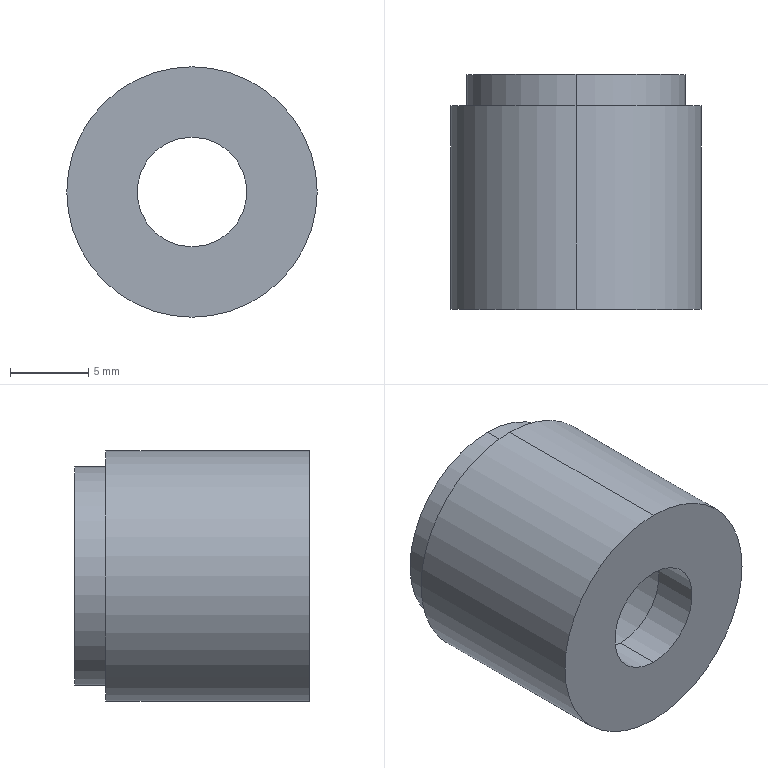Part | STEP file | Generic block | 1 solid | 12 faces | box 16 x 15 x 16 mm | volume 1666 mm3 | cylinder 8 | plane 4 | commonest cylinder face diameters 7 x2 11 x2 14 x2 16 x2
STEP:
#1=CARTESIAN_POINT('',(0.,0.,0.));
#2=DIRECTION('',(0.,0.,1.));
#3=DIRECTION('',(1.,0.,0.));
#4=AXIS2_PLACEMENT_3D('',#1,#2,#3);
#5=CARTESIAN_POINT('',(3.5,3.,5.5));
#6=VERTEX_POINT('',#5);
#7=CARTESIAN_POINT('',(3.5,15.,5.5));
#8=VERTEX_POINT('',#7);
#9=CARTESIAN_POINT('',(3.5,3.,5.5));
#10=DIRECTION('',(0.,1.,0.));
#11=VECTOR('',#10,1.);
#12=LINE('',#9,#11);
#13=CARTESIAN_POINT('',(3.5,3.,0.));
#14=DIRECTION('',(0.,1.,0.));
#15=DIRECTION('',(0.,0.,1.));
#16=AXIS2_PLACEMENT_3D('',#13,#14,#15);
#17=CYLINDRICAL_SURFACE('',#16,5.5);
#18=CARTESIAN_POINT('',(6.283,0.));
#19=DIRECTION('',(0.,1.));
#20=VECTOR('',#19,1.);
#21=LINE('',#18,#20);
#22=(GEOMETRIC_REPRESENTATION_CONTEXT(2)PARAMETRIC_REPRESENTATION_CONTEXT()REPRESENTATION_CONTEXT('',''));
#23=DEFINITIONAL_REPRESENTATION('',(#21),#22);
#24=PCURVE('',#17,#23);
#25=CARTESIAN_POINT('',(3.5,3.,0.));
#26=DIRECTION('',(0.,1.,0.));
#27=DIRECTION('',(0.,0.,1.));
#28=AXIS2_PLACEMENT_3D('',#25,#26,#27);
#29=CYLINDRICAL_SURFACE('',#28,5.5);
#30=CARTESIAN_POINT('',(0.,0.));
#31=DIRECTION('',(0.,1.));
#32=VECTOR('',#31,1.);
#33=LINE('',#30,#32);
#34=(GEOMETRIC_REPRESENTATION_CONTEXT(2)PARAMETRIC_REPRESENTATION_CONTEXT()REPRESENTATION_CONTEXT('',''));
#35=DEFINITIONAL_REPRESENTATION('',(#33),#34);
#36=PCURVE('',#29,#35);
#37=SURFACE_CURVE('',#12,(#24,#36),.PCURVE_S1.);
#38=EDGE_CURVE('',#6,#8,#37,.T.);
#39=ORIENTED_EDGE('',*,*,#38,.T.);
#40=CARTESIAN_POINT('',(3.5,15.,-5.5));
#41=VERTEX_POINT('',#40);
#42=CARTESIAN_POINT('',(3.5,15.,0.));
#43=DIRECTION('',(0.,1.,0.));
#44=DIRECTION('',(0.,0.,1.));
#45=AXIS2_PLACEMENT_3D('',#42,#43,#44);
#46=CIRCLE('',#45,5.5);
#47=CARTESIAN_POINT('',(0.,12.));
#48=DIRECTION('',(1.,0.));
#49=VECTOR('',#48,1.);
#50=LINE('',#47,#49);
#51=(GEOMETRIC_REPRESENTATION_CONTEXT(2)PARAMETRIC_REPRESENTATION_CONTEXT()REPRESENTATION_CONTEXT('',''));
#52=DEFINITIONAL_REPRESENTATION('',(#50),#51);
#53=PCURVE('',#17,#52);
#54=CARTESIAN_POINT('',(-3.5,15.,0.));
#55=DIRECTION('',(0.,-1.,0.));
#56=DIRECTION('',(0.,0.,-1.));
#57=AXIS2_PLACEMENT_3D('',#54,#55,#56);
#58=PLANE('',#57);
#59=CARTESIAN_POINT('',(-5.5,7.));
#60=CARTESIAN_POINT('',(-5.5,16.526));
#61=CARTESIAN_POINT('',(2.75,11.763));
#62=CARTESIAN_POINT('',(11.,7.));
#63=CARTESIAN_POINT('',(2.75,2.237));
#64=CARTESIAN_POINT('',(-5.5,-2.526));
#65=CARTESIAN_POINT('',(-5.5,7.));
#66=(BOUNDED_CURVE()B_SPLINE_CURVE(2,(#59,#60,#61,#62,#63,#64,#65),.UNSPECIFIED.,.T.,.F.)B_SPLINE_CURVE_WITH_KNOTS((1,2,2,2,2,1),(-2.094,0.,2.094,4.189,6.283,8.378),.UNSPECIFIED.)CURVE()GEOMETRIC_REPRESENTATION_ITEM()RATIONAL_B_SPLINE_CURVE((1.,0.5,1.,0.5,1.,0.5,1.))REPRESENTATION_ITEM(''));
#67=(GEOMETRIC_REPRESENTATION_CONTEXT(2)PARAMETRIC_REPRESENTATION_CONTEXT()REPRESENTATION_CONTEXT('',''));
#68=DEFINITIONAL_REPRESENTATION('',(#66),#67);
#69=PCURVE('',#58,#68);
#70=SURFACE_CURVE('',#46,(#53,#69),.PCURVE_S1.);
#71=EDGE_CURVE('',#41,#8,#70,.T.);
#72=ORIENTED_EDGE('',*,*,#71,.F.);
#73=CARTESIAN_POINT('',(3.5,3.,-5.5));
#74=VERTEX_POINT('',#73);
#75=CARTESIAN_POINT('',(3.5,3.,-5.5));
#76=DIRECTION('',(0.,1.,0.));
#77=VECTOR('',#76,1.);
#78=LINE('',#75,#77);
#79=CARTESIAN_POINT('',(3.142,0.));
#80=DIRECTION('',(0.,1.));
#81=VECTOR('',#80,1.);
#82=LINE('',#79,#81);
#83=(GEOMETRIC_REPRESENTATION_CONTEXT(2)PARAMETRIC_REPRESENTATION_CONTEXT()REPRESENTATION_CONTEXT('',''));
#84=DEFINITIONAL_REPRESENTATION('',(#82),#83);
#85=PCURVE('',#17,#84);
#86=CARTESIAN_POINT('',(3.142,0.));
#87=DIRECTION('',(0.,1.));
#88=VECTOR('',#87,1.);
#89=LINE('',#86,#88);
#90=(GEOMETRIC_REPRESENTATION_CONTEXT(2)PARAMETRIC_REPRESENTATION_CONTEXT()REPRESENTATION_CONTEXT('',''));
#91=DEFINITIONAL_REPRESENTATION('',(#89),#90);
#92=PCURVE('',#29,#91);
#93=SURFACE_CURVE('',#78,(#85,#92),.PCURVE_S1.);
#94=EDGE_CURVE('',#74,#41,#93,.T.);
#95=ORIENTED_EDGE('',*,*,#94,.F.);
#96=CARTESIAN_POINT('',(3.5,3.,0.));
#97=DIRECTION('',(0.,1.,0.));
#98=DIRECTION('',(0.,0.,1.));
#99=AXIS2_PLACEMENT_3D('',#96,#97,#98);
#100=CIRCLE('',#99,5.5);
#101=CARTESIAN_POINT('',(0.,0.));
#102=DIRECTION('',(1.,0.));
#103=VECTOR('',#102,1.);
#104=LINE('',#101,#103);
#105=(GEOMETRIC_REPRESENTATION_CONTEXT(2)PARAMETRIC_REPRESENTATION_CONTEXT()REPRESENTATION_CONTEXT('',''));
#106=DEFINITIONAL_REPRESENTATION('',(#104),#105);
#107=PCURVE('',#17,#106);
#108=CARTESIAN_POINT('',(3.5,3.,0.));
#109=DIRECTION('',(0.,1.,0.));
#110=DIRECTION('',(0.,0.,1.));
#111=AXIS2_PLACEMENT_3D('',#108,#109,#110);
#112=PLANE('',#111);
#113=CARTESIAN_POINT('',(0.,0.));
#114=DIRECTION('',(1.,0.));
#115=AXIS2_PLACEMENT_2D('',#113,#114);
#116=CIRCLE('',#115,5.5);
#117=(GEOMETRIC_REPRESENTATION_CONTEXT(2)PARAMETRIC_REPRESENTATION_CONTEXT()REPRESENTATION_CONTEXT('',''));
#118=DEFINITIONAL_REPRESENTATION('',(#116),#117);
#119=PCURVE('',#112,#118);
#120=SURFACE_CURVE('',#100,(#107,#119),.PCURVE_S1.);
#121=EDGE_CURVE('',#74,#6,#120,.T.);
#122=ORIENTED_EDGE('',*,*,#121,.T.);
#123=EDGE_LOOP('',(#39,#72,#95,#122));
#124=FACE_BOUND('',#123,.F.);
#125=ADVANCED_FACE('',(#124),#17,.F.);
#126=CARTESIAN_POINT('',(3.5,15.,-7.));
#127=VERTEX_POINT('',#126);
#128=CARTESIAN_POINT('',(3.5,15.,7.));
#129=VERTEX_POINT('',#128);
#130=CARTESIAN_POINT('',(3.5,15.,0.));
#131=DIRECTION('',(0.,-1.,0.));
#132=DIRECTION('',(0.,0.,-1.));
#133=AXIS2_PLACEMENT_3D('',#130,#131,#132);
#134=CIRCLE('',#133,7.);
#135=CARTESIAN_POINT('',(3.5,0.,0.));
#136=DIRECTION('',(0.,-1.,0.));
#137=DIRECTION('',(0.,0.,-1.));
#138=AXIS2_PLACEMENT_3D('',#135,#136,#137);
#139=CYLINDRICAL_SURFACE('',#138,7.);
#140=CARTESIAN_POINT('',(0.,-15.));
#141=DIRECTION('',(1.,0.));
#142=VECTOR('',#141,1.);
#143=LINE('',#140,#142);
#144=(GEOMETRIC_REPRESENTATION_CONTEXT(2)PARAMETRIC_REPRESENTATION_CONTEXT()REPRESENTATION_CONTEXT('',''));
#145=DEFINITIONAL_REPRESENTATION('',(#143),#144);
#146=PCURVE('',#139,#145);
#147=CARTESIAN_POINT('',(0.,7.));
#148=DIRECTION('',(1.,0.));
#149=AXIS2_PLACEMENT_2D('',#147,#148);
#150=CIRCLE('',#149,7.);
#151=(GEOMETRIC_REPRESENTATION_CONTEXT(2)PARAMETRIC_REPRESENTATION_CONTEXT()REPRESENTATION_CONTEXT('',''));
#152=DEFINITIONAL_REPRESENTATION('',(#150),#151);
#153=PCURVE('',#58,#152);
#154=SURFACE_CURVE('',#134,(#146,#153),.PCURVE_S1.);
#155=EDGE_CURVE('',#127,#129,#154,.T.);
#156=ORIENTED_EDGE('',*,*,#155,.T.);
#157=CARTESIAN_POINT('',(3.5,13.,7.));
#158=VERTEX_POINT('',#157);
#159=CARTESIAN_POINT('',(3.5,0.,7.));
#160=DIRECTION('',(0.,-1.,0.));
#161=VECTOR('',#160,1.);
#162=LINE('',#159,#161);
#163=CARTESIAN_POINT('',(3.142,0.));
#164=DIRECTION('',(0.,1.));
#165=VECTOR('',#164,1.);
#166=LINE('',#163,#165);
#167=(GEOMETRIC_REPRESENTATION_CONTEXT(2)PARAMETRIC_REPRESENTATION_CONTEXT()REPRESENTATION_CONTEXT('',''));
#168=DEFINITIONAL_REPRESENTATION('',(#166),#167);
#169=PCURVE('',#139,#168);
#170=CARTESIAN_POINT('',(3.5,0.,0.));
#171=DIRECTION('',(0.,-1.,0.));
#172=DIRECTION('',(0.,0.,-1.));
#173=AXIS2_PLACEMENT_3D('',#170,#171,#172);
#174=CYLINDRICAL_SURFACE('',#173,7.);
#175=CARTESIAN_POINT('',(3.142,0.));
#176=DIRECTION('',(0.,1.));
#177=VECTOR('',#176,1.);
#178=LINE('',#175,#177);
#179=(GEOMETRIC_REPRESENTATION_CONTEXT(2)PARAMETRIC_REPRESENTATION_CONTEXT()REPRESENTATION_CONTEXT('',''));
#180=DEFINITIONAL_REPRESENTATION('',(#178),#179);
#181=PCURVE('',#174,#180);
#182=SURFACE_CURVE('',#162,(#169,#181),.PCURVE_S1.);
#183=EDGE_CURVE('',#129,#158,#182,.T.);
#184=ORIENTED_EDGE('',*,*,#183,.T.);
#185=CARTESIAN_POINT('',(3.5,13.,-7.));
#186=VERTEX_POINT('',#185);
#187=CARTESIAN_POINT('',(3.5,13.,0.));
#188=DIRECTION('',(0.,-1.,0.));
#189=DIRECTION('',(0.,0.,-1.));
#190=AXIS2_PLACEMENT_3D('',#187,#188,#189);
#191=CIRCLE('',#190,7.);
#192=CARTESIAN_POINT('',(0.,-13.));
#193=DIRECTION('',(1.,0.));
#194=VECTOR('',#193,1.);
#195=LINE('',#192,#194);
#196=(GEOMETRIC_REPRESENTATION_CONTEXT(2)PARAMETRIC_REPRESENTATION_CONTEXT()REPRESENTATION_CONTEXT('',''));
#197=DEFINITIONAL_REPRESENTATION('',(#195),#196);
#198=PCURVE('',#139,#197);
#199=CARTESIAN_POINT('',(-4.5,13.,0.));
#200=DIRECTION('',(0.,-1.,0.));
#201=DIRECTION('',(0.,0.,-1.));
#202=AXIS2_PLACEMENT_3D('',#199,#200,#201);
#203=PLANE('',#202);
#204=CARTESIAN_POINT('',(0.,8.));
#205=DIRECTION('',(1.,0.));
#206=AXIS2_PLACEMENT_2D('',#204,#205);
#207=CIRCLE('',#206,7.);
#208=(GEOMETRIC_REPRESENTATION_CONTEXT(2)PARAMETRIC_REPRESENTATION_CONTEXT()REPRESENTATION_CONTEXT('',''));
#209=DEFINITIONAL_REPRESENTATION('',(#207),#208);
#210=PCURVE('',#203,#209);
#211=SURFACE_CURVE('',#191,(#198,#210),.PCURVE_S1.);
#212=EDGE_CURVE('',#186,#158,#211,.T.);
#213=ORIENTED_EDGE('',*,*,#212,.F.);
#214=CARTESIAN_POINT('',(3.5,0.,-7.));
#215=DIRECTION('',(0.,-1.,0.));
#216=VECTOR('',#215,1.);
#217=LINE('',#214,#216);
#218=CARTESIAN_POINT('',(0.,0.));
#219=DIRECTION('',(0.,1.));
#220=VECTOR('',#219,1.);
#221=LINE('',#218,#220);
#222=(GEOMETRIC_REPRESENTATION_CONTEXT(2)PARAMETRIC_REPRESENTATION_CONTEXT()REPRESENTATION_CONTEXT('',''));
#223=DEFINITIONAL_REPRESENTATION('',(#221),#222);
#224=PCURVE('',#139,#223);
#225=CARTESIAN_POINT('',(6.283,0.));
#226=DIRECTION('',(0.,1.));
#227=VECTOR('',#226,1.);
#228=LINE('',#225,#227);
#229=(GEOMETRIC_REPRESENTATION_CONTEXT(2)PARAMETRIC_REPRESENTATION_CONTEXT()REPRESENTATION_CONTEXT('',''));
#230=DEFINITIONAL_REPRESENTATION('',(#228),#229);
#231=PCURVE('',#174,#230);
#232=SURFACE_CURVE('',#217,(#224,#231),.PCURVE_S1.);
#233=EDGE_CURVE('',#127,#186,#232,.T.);
#234=ORIENTED_EDGE('',*,*,#233,.F.);
#235=EDGE_LOOP('',(#156,#184,#213,#234));
#236=FACE_BOUND('',#235,.T.);
#237=ADVANCED_FACE('',(#236),#139,.T.);
#238=CARTESIAN_POINT('',(3.5,13.,-8.));
#239=VERTEX_POINT('',#238);
#240=CARTESIAN_POINT('',(3.5,13.,8.));
#241=VERTEX_POINT('',#240);
#242=CARTESIAN_POINT('',(3.5,13.,0.));
#243=DIRECTION('',(0.,-1.,0.));
#244=DIRECTION('',(0.,0.,-1.));
#245=AXIS2_PLACEMENT_3D('',#242,#243,#244);
#246=CIRCLE('',#245,8.);
#247=CARTESIAN_POINT('',(3.5,0.,0.));
#248=DIRECTION('',(0.,-1.,0.));
#249=DIRECTION('',(0.,0.,-1.));
#250=AXIS2_PLACEMENT_3D('',#247,#248,#249);
#251=CYLINDRICAL_SURFACE('',#250,8.);
#252=CARTESIAN_POINT('',(0.,-13.));
#253=DIRECTION('',(1.,0.));
#254=VECTOR('',#253,1.);
#255=LINE('',#252,#254);
#256=(GEOMETRIC_REPRESENTATION_CONTEXT(2)PARAMETRIC_REPRESENTATION_CONTEXT()REPRESENTATION_CONTEXT('',''));
#257=DEFINITIONAL_REPRESENTATION('',(#255),#256);
#258=PCURVE('',#251,#257);
#259=CARTESIAN_POINT('',(0.,8.));
#260=DIRECTION('',(1.,0.));
#261=AXIS2_PLACEMENT_2D('',#259,#260);
#262=CIRCLE('',#261,8.);
#263=(GEOMETRIC_REPRESENTATION_CONTEXT(2)PARAMETRIC_REPRESENTATION_CONTEXT()REPRESENTATION_CONTEXT('',''));
#264=DEFINITIONAL_REPRESENTATION('',(#262),#263);
#265=PCURVE('',#203,#264);
#266=SURFACE_CURVE('',#246,(#258,#265),.PCURVE_S1.);
#267=EDGE_CURVE('',#239,#241,#266,.T.);
#268=ORIENTED_EDGE('',*,*,#267,.T.);
#269=CARTESIAN_POINT('',(3.5,0.,8.));
#270=VERTEX_POINT('',#269);
#271=CARTESIAN_POINT('',(3.5,0.,8.));
#272=DIRECTION('',(0.,-1.,0.));
#273=VECTOR('',#272,1.);
#274=LINE('',#271,#273);
#275=CARTESIAN_POINT('',(3.142,0.));
#276=DIRECTION('',(0.,1.));
#277=VECTOR('',#276,1.);
#278=LINE('',#275,#277);
#279=(GEOMETRIC_REPRESENTATION_CONTEXT(2)PARAMETRIC_REPRESENTATION_CONTEXT()REPRESENTATION_CONTEXT('',''));
#280=DEFINITIONAL_REPRESENTATION('',(#278),#279);
#281=PCURVE('',#251,#280);
#282=CARTESIAN_POINT('',(3.5,0.,0.));
#283=DIRECTION('',(0.,-1.,0.));
#284=DIRECTION('',(0.,0.,-1.));
#285=AXIS2_PLACEMENT_3D('',#282,#283,#284);
#286=CYLINDRICAL_SURFACE('',#285,8.);
#287=CARTESIAN_POINT('',(3.142,0.));
#288=DIRECTION('',(0.,1.));
#289=VECTOR('',#288,1.);
#290=LINE('',#287,#289);
#291=(GEOMETRIC_REPRESENTATION_CONTEXT(2)PARAMETRIC_REPRESENTATION_CONTEXT()REPRESENTATION_CONTEXT('',''));
#292=DEFINITIONAL_REPRESENTATION('',(#290),#291);
#293=PCURVE('',#286,#292);
#294=SURFACE_CURVE('',#274,(#281,#293),.PCURVE_S1.);
#295=EDGE_CURVE('',#241,#270,#294,.T.);
#296=ORIENTED_EDGE('',*,*,#295,.T.);
#297=CARTESIAN_POINT('',(3.5,0.,-8.));
#298=VERTEX_POINT('',#297);
#299=CARTESIAN_POINT('',(3.5,0.,0.));
#300=DIRECTION('',(0.,-1.,0.));
#301=DIRECTION('',(0.,0.,-1.));
#302=AXIS2_PLACEMENT_3D('',#299,#300,#301);
#303=CIRCLE('',#302,8.);
#304=CARTESIAN_POINT('',(0.,0.));
#305=DIRECTION('',(1.,0.));
#306=VECTOR('',#305,1.);
#307=LINE('',#304,#306);
#308=(GEOMETRIC_REPRESENTATION_CONTEXT(2)PARAMETRIC_REPRESENTATION_CONTEXT()REPRESENTATION_CONTEXT('',''));
#309=DEFINITIONAL_REPRESENTATION('',(#307),#308);
#310=PCURVE('',#251,#309);
#311=CARTESIAN_POINT('',(0.,0.,0.));
#312=DIRECTION('',(0.,1.,0.));
#313=DIRECTION('',(0.,0.,1.));
#314=AXIS2_PLACEMENT_3D('',#311,#312,#313);
#315=PLANE('',#314);
#316=CARTESIAN_POINT('',(-8.,3.5));
#317=CARTESIAN_POINT('',(-8.,17.356));
#318=CARTESIAN_POINT('',(4.,10.428));
#319=CARTESIAN_POINT('',(16.,3.5));
#320=CARTESIAN_POINT('',(4.,-3.428));
#321=CARTESIAN_POINT('',(-8.,-10.356));
#322=CARTESIAN_POINT('',(-8.,3.5));
#323=(BOUNDED_CURVE()B_SPLINE_CURVE(2,(#316,#317,#318,#319,#320,#321,#322),.UNSPECIFIED.,.T.,.F.)B_SPLINE_CURVE_WITH_KNOTS((1,2,2,2,2,1),(-2.094,0.,2.094,4.189,6.283,8.378),.UNSPECIFIED.)CURVE()GEOMETRIC_REPRESENTATION_ITEM()RATIONAL_B_SPLINE_CURVE((1.,0.5,1.,0.5,1.,0.5,1.))REPRESENTATION_ITEM(''));
#324=(GEOMETRIC_REPRESENTATION_CONTEXT(2)PARAMETRIC_REPRESENTATION_CONTEXT()REPRESENTATION_CONTEXT('',''));
#325=DEFINITIONAL_REPRESENTATION('',(#323),#324);
#326=PCURVE('',#315,#325);
#327=SURFACE_CURVE('',#303,(#310,#326),.PCURVE_S1.);
#328=EDGE_CURVE('',#298,#270,#327,.T.);
#329=ORIENTED_EDGE('',*,*,#328,.F.);
#330=CARTESIAN_POINT('',(3.5,0.,-8.));
#331=DIRECTION('',(0.,-1.,0.));
#332=VECTOR('',#331,1.);
#333=LINE('',#330,#332);
#334=CARTESIAN_POINT('',(0.,0.));
#335=DIRECTION('',(0.,1.));
#336=VECTOR('',#335,1.);
#337=LINE('',#334,#336);
#338=(GEOMETRIC_REPRESENTATION_CONTEXT(2)PARAMETRIC_REPRESENTATION_CONTEXT()REPRESENTATION_CONTEXT('',''));
#339=DEFINITIONAL_REPRESENTATION('',(#337),#338);
#340=PCURVE('',#251,#339);
#341=CARTESIAN_POINT('',(6.283,0.));
#342=DIRECTION('',(0.,1.));
#343=VECTOR('',#342,1.);
#344=LINE('',#341,#343);
#345=(GEOMETRIC_REPRESENTATION_CONTEXT(2)PARAMETRIC_REPRESENTATION_CONTEXT()REPRESENTATION_CONTEXT('',''));
#346=DEFINITIONAL_REPRESENTATION('',(#344),#345);
#347=PCURVE('',#286,#346);
#348=SURFACE_CURVE('',#333,(#340,#347),.PCURVE_S1.);
#349=EDGE_CURVE('',#239,#298,#348,.T.);
#350=ORIENTED_EDGE('',*,*,#349,.F.);
#351=EDGE_LOOP('',(#268,#296,#329,#350));
#352=FACE_BOUND('',#351,.T.);
#353=ADVANCED_FACE('',(#352),#251,.T.);
#354=CARTESIAN_POINT('',(3.5,3.,-3.5));
#355=VERTEX_POINT('',#354);
#356=CARTESIAN_POINT('',(3.5,0.,-3.5));
#357=VERTEX_POINT('',#356);
#358=CARTESIAN_POINT('',(3.5,0.,-3.5));
#359=DIRECTION('',(0.,-1.,0.));
#360=VECTOR('',#359,1.);
#361=LINE('',#358,#360);
#362=CARTESIAN_POINT('',(3.5,0.,0.));
#363=DIRECTION('',(0.,-1.,0.));
#364=DIRECTION('',(0.,0.,-1.));
#365=AXIS2_PLACEMENT_3D('',#362,#363,#364);
#366=CYLINDRICAL_SURFACE('',#365,3.5);
#367=CARTESIAN_POINT('',(6.283,0.));
#368=DIRECTION('',(0.,1.));
#369=VECTOR('',#368,1.);
#370=LINE('',#367,#369);
#371=(GEOMETRIC_REPRESENTATION_CONTEXT(2)PARAMETRIC_REPRESENTATION_CONTEXT()REPRESENTATION_CONTEXT('',''));
#372=DEFINITIONAL_REPRESENTATION('',(#370),#371);
#373=PCURVE('',#366,#372);
#374=CARTESIAN_POINT('',(3.5,0.,0.));
#375=DIRECTION('',(0.,-1.,0.));
#376=DIRECTION('',(0.,0.,-1.));
#377=AXIS2_PLACEMENT_3D('',#374,#375,#376);
#378=CYLINDRICAL_SURFACE('',#377,3.5);
#379=CARTESIAN_POINT('',(0.,0.));
#380=DIRECTION('',(0.,1.));
#381=VECTOR('',#380,1.);
#382=LINE('',#379,#381);
#383=(GEOMETRIC_REPRESENTATION_CONTEXT(2)PARAMETRIC_REPRESENTATION_CONTEXT()REPRESENTATION_CONTEXT('',''));
#384=DEFINITIONAL_REPRESENTATION('',(#382),#383);
#385=PCURVE('',#378,#384);
#386=SURFACE_CURVE('',#361,(#373,#385),.PCURVE_S1.);
#387=EDGE_CURVE('',#355,#357,#386,.T.);
#388=ORIENTED_EDGE('',*,*,#387,.T.);
#389=CARTESIAN_POINT('',(3.5,0.,3.5));
#390=VERTEX_POINT('',#389);
#391=CARTESIAN_POINT('',(3.5,0.,0.));
#392=DIRECTION('',(0.,-1.,0.));
#393=DIRECTION('',(0.,0.,-1.));
#394=AXIS2_PLACEMENT_3D('',#391,#392,#393);
#395=CIRCLE('',#394,3.5);
#396=CARTESIAN_POINT('',(0.,0.));
#397=DIRECTION('',(1.,0.));
#398=VECTOR('',#397,1.);
#399=LINE('',#396,#398);
#400=(GEOMETRIC_REPRESENTATION_CONTEXT(2)PARAMETRIC_REPRESENTATION_CONTEXT()REPRESENTATION_CONTEXT('',''));
#401=DEFINITIONAL_REPRESENTATION('',(#399),#400);
#402=PCURVE('',#366,#401);
#403=CARTESIAN_POINT('',(-3.5,3.5));
#404=CARTESIAN_POINT('',(-3.5,9.562));
#405=CARTESIAN_POINT('',(1.75,6.531));
#406=CARTESIAN_POINT('',(7.,3.5));
#407=CARTESIAN_POINT('',(1.75,0.4689));
#408=CARTESIAN_POINT('',(-3.5,-2.562));
#409=CARTESIAN_POINT('',(-3.5,3.5));
#410=(BOUNDED_CURVE()B_SPLINE_CURVE(2,(#403,#404,#405,#406,#407,#408,#409),.UNSPECIFIED.,.T.,.F.)B_SPLINE_CURVE_WITH_KNOTS((1,2,2,2,2,1),(-2.094,0.,2.094,4.189,6.283,8.378),.UNSPECIFIED.)CURVE()GEOMETRIC_REPRESENTATION_ITEM()RATIONAL_B_SPLINE_CURVE((1.,0.5,1.,0.5,1.,0.5,1.))REPRESENTATION_ITEM(''));
#411=(GEOMETRIC_REPRESENTATION_CONTEXT(2)PARAMETRIC_REPRESENTATION_CONTEXT()REPRESENTATION_CONTEXT('',''));
#412=DEFINITIONAL_REPRESENTATION('',(#410),#411);
#413=PCURVE('',#315,#412);
#414=SURFACE_CURVE('',#395,(#402,#413),.PCURVE_S1.);
#415=EDGE_CURVE('',#390,#357,#414,.T.);
#416=ORIENTED_EDGE('',*,*,#415,.F.);
#417=CARTESIAN_POINT('',(3.5,3.,3.5));
#418=VERTEX_POINT('',#417);
#419=CARTESIAN_POINT('',(3.5,0.,3.5));
#420=DIRECTION('',(0.,-1.,0.));
#421=VECTOR('',#420,1.);
#422=LINE('',#419,#421);
#423=CARTESIAN_POINT('',(3.142,0.));
#424=DIRECTION('',(0.,1.));
#425=VECTOR('',#424,1.);
#426=LINE('',#423,#425);
#427=(GEOMETRIC_REPRESENTATION_CONTEXT(2)PARAMETRIC_REPRESENTATION_CONTEXT()REPRESENTATION_CONTEXT('',''));
#428=DEFINITIONAL_REPRESENTATION('',(#426),#427);
#429=PCURVE('',#366,#428);
#430=CARTESIAN_POINT('',(3.142,0.));
#431=DIRECTION('',(0.,1.));
#432=VECTOR('',#431,1.);
#433=LINE('',#430,#432);
#434=(GEOMETRIC_REPRESENTATION_CONTEXT(2)PARAMETRIC_REPRESENTATION_CONTEXT()REPRESENTATION_CONTEXT('',''));
#435=DEFINITIONAL_REPRESENTATION('',(#433),#434);
#436=PCURVE('',#378,#435);
#437=SURFACE_CURVE('',#422,(#429,#436),.PCURVE_S1.);
#438=EDGE_CURVE('',#418,#390,#437,.T.);
#439=ORIENTED_EDGE('',*,*,#438,.F.);
#440=CARTESIAN_POINT('',(3.5,3.,0.));
#441=DIRECTION('',(0.,-1.,0.));
#442=DIRECTION('',(0.,0.,1.));
#443=AXIS2_PLACEMENT_3D('',#440,#441,#442);
#444=CIRCLE('',#443,3.5);
#445=CARTESIAN_POINT('',(3.142,-3.));
#446=DIRECTION('',(1.,0.));
#447=VECTOR('',#446,1.);
#448=LINE('',#445,#447);
#449=(GEOMETRIC_REPRESENTATION_CONTEXT(2)PARAMETRIC_REPRESENTATION_CONTEXT()REPRESENTATION_CONTEXT('',''));
#450=DEFINITIONAL_REPRESENTATION('',(#448),#449);
#451=PCURVE('',#366,#450);
#452=CARTESIAN_POINT('',(3.5,0.));
#453=CARTESIAN_POINT('',(3.5,-6.062));
#454=CARTESIAN_POINT('',(-1.75,-3.031));
#455=CARTESIAN_POINT('',(-7.,0.));
#456=CARTESIAN_POINT('',(-1.75,3.031));
#457=CARTESIAN_POINT('',(3.5,6.062));
#458=CARTESIAN_POINT('',(3.5,0.));
#459=(BOUNDED_CURVE()B_SPLINE_CURVE(2,(#452,#453,#454,#455,#456,#457,#458),.UNSPECIFIED.,.T.,.F.)B_SPLINE_CURVE_WITH_KNOTS((1,2,2,2,2,1),(-2.094,0.,2.094,4.189,6.283,8.378),.UNSPECIFIED.)CURVE()GEOMETRIC_REPRESENTATION_ITEM()RATIONAL_B_SPLINE_CURVE((1.,0.5,1.,0.5,1.,0.5,1.))REPRESENTATION_ITEM(''));
#460=(GEOMETRIC_REPRESENTATION_CONTEXT(2)PARAMETRIC_REPRESENTATION_CONTEXT()REPRESENTATION_CONTEXT('',''));
#461=DEFINITIONAL_REPRESENTATION('',(#459),#460);
#462=PCURVE('',#112,#461);
#463=SURFACE_CURVE('',#444,(#451,#462),.PCURVE_S1.);
#464=EDGE_CURVE('',#418,#355,#463,.T.);
#465=ORIENTED_EDGE('',*,*,#464,.T.);
#466=EDGE_LOOP('',(#388,#416,#439,#465));
#467=FACE_BOUND('',#466,.F.);
#468=ADVANCED_FACE('',(#467),#366,.F.);
#469=CARTESIAN_POINT('',(3.5,0.,0.));
#470=DIRECTION('',(0.,-1.,0.));
#471=DIRECTION('',(0.,0.,-1.));
#472=AXIS2_PLACEMENT_3D('',#469,#470,#471);
#473=CIRCLE('',#472,3.5);
#474=CARTESIAN_POINT('',(0.,0.));
#475=DIRECTION('',(1.,0.));
#476=VECTOR('',#475,1.);
#477=LINE('',#474,#476);
#478=(GEOMETRIC_REPRESENTATION_CONTEXT(2)PARAMETRIC_REPRESENTATION_CONTEXT()REPRESENTATION_CONTEXT('',''));
#479=DEFINITIONAL_REPRESENTATION('',(#477),#478);
#480=PCURVE('',#378,#479);
#481=CARTESIAN_POINT('',(-3.5,3.5));
#482=CARTESIAN_POINT('',(-3.5,9.562));
#483=CARTESIAN_POINT('',(1.75,6.531));
#484=CARTESIAN_POINT('',(7.,3.5));
#485=CARTESIAN_POINT('',(1.75,0.4689));
#486=CARTESIAN_POINT('',(-3.5,-2.562));
#487=CARTESIAN_POINT('',(-3.5,3.5));
#488=(BOUNDED_CURVE()B_SPLINE_CURVE(2,(#481,#482,#483,#484,#485,#486,#487),.UNSPECIFIED.,.T.,.F.)B_SPLINE_CURVE_WITH_KNOTS((1,2,2,2,2,1),(-2.094,0.,2.094,4.189,6.283,8.378),.UNSPECIFIED.)CURVE()GEOMETRIC_REPRESENTATION_ITEM()RATIONAL_B_SPLINE_CURVE((1.,0.5,1.,0.5,1.,0.5,1.))REPRESENTATION_ITEM(''));
#489=(GEOMETRIC_REPRESENTATION_CONTEXT(2)PARAMETRIC_REPRESENTATION_CONTEXT()REPRESENTATION_CONTEXT('',''));
#490=DEFINITIONAL_REPRESENTATION('',(#488),#489);
#491=PCURVE('',#315,#490);
#492=SURFACE_CURVE('',#473,(#480,#491),.PCURVE_S1.);
#493=EDGE_CURVE('',#357,#390,#492,.T.);
#494=ORIENTED_EDGE('',*,*,#493,.F.);
#495=ORIENTED_EDGE('',*,*,#387,.F.);
#496=CARTESIAN_POINT('',(3.5,3.,0.));
#497=DIRECTION('',(0.,-1.,0.));
#498=DIRECTION('',(0.,0.,1.));
#499=AXIS2_PLACEMENT_3D('',#496,#497,#498);
#500=CIRCLE('',#499,3.5);
#501=CARTESIAN_POINT('',(-3.142,-3.));
#502=DIRECTION('',(1.,0.));
#503=VECTOR('',#502,1.);
#504=LINE('',#501,#503);
#505=(GEOMETRIC_REPRESENTATION_CONTEXT(2)PARAMETRIC_REPRESENTATION_CONTEXT()REPRESENTATION_CONTEXT('',''));
#506=DEFINITIONAL_REPRESENTATION('',(#504),#505);
#507=PCURVE('',#378,#506);
#508=CARTESIAN_POINT('',(3.5,0.));
#509=CARTESIAN_POINT('',(3.5,-6.062));
#510=CARTESIAN_POINT('',(-1.75,-3.031));
#511=CARTESIAN_POINT('',(-7.,0.));
#512=CARTESIAN_POINT('',(-1.75,3.031));
#513=CARTESIAN_POINT('',(3.5,6.062));
#514=CARTESIAN_POINT('',(3.5,0.));
#515=(BOUNDED_CURVE()B_SPLINE_CURVE(2,(#508,#509,#510,#511,#512,#513,#514),.UNSPECIFIED.,.T.,.F.)B_SPLINE_CURVE_WITH_KNOTS((1,2,2,2,2,1),(-2.094,0.,2.094,4.189,6.283,8.378),.UNSPECIFIED.)CURVE()GEOMETRIC_REPRESENTATION_ITEM()RATIONAL_B_SPLINE_CURVE((1.,0.5,1.,0.5,1.,0.5,1.))REPRESENTATION_ITEM(''));
#516=(GEOMETRIC_REPRESENTATION_CONTEXT(2)PARAMETRIC_REPRESENTATION_CONTEXT()REPRESENTATION_CONTEXT('',''));
#517=DEFINITIONAL_REPRESENTATION('',(#515),#516);
#518=PCURVE('',#112,#517);
#519=SURFACE_CURVE('',#500,(#507,#518),.PCURVE_S1.);
#520=EDGE_CURVE('',#355,#418,#519,.T.);
#521=ORIENTED_EDGE('',*,*,#520,.T.);
#522=ORIENTED_EDGE('',*,*,#438,.T.);
#523=EDGE_LOOP('',(#494,#495,#521,#522));
#524=FACE_BOUND('',#523,.F.);
#525=ADVANCED_FACE('',(#524),#378,.F.);
#526=ORIENTED_EDGE('',*,*,#493,.F.);
#527=ORIENTED_EDGE('',*,*,#415,.F.);
#528=EDGE_LOOP('',(#526,#527));
#529=FACE_BOUND('',#528,.T.);
#530=ORIENTED_EDGE('',*,*,#328,.T.);
#531=CARTESIAN_POINT('',(3.5,0.,0.));
#532=DIRECTION('',(0.,-1.,0.));
#533=DIRECTION('',(0.,0.,-1.));
#534=AXIS2_PLACEMENT_3D('',#531,#532,#533);
#535=CIRCLE('',#534,8.);
#536=CARTESIAN_POINT('',(-8.,3.5));
#537=CARTESIAN_POINT('',(-8.,17.356));
#538=CARTESIAN_POINT('',(4.,10.428));
#539=CARTESIAN_POINT('',(16.,3.5));
#540=CARTESIAN_POINT('',(4.,-3.428));
#541=CARTESIAN_POINT('',(-8.,-10.356));
#542=CARTESIAN_POINT('',(-8.,3.5));
#543=(BOUNDED_CURVE()B_SPLINE_CURVE(2,(#536,#537,#538,#539,#540,#541,#542),.UNSPECIFIED.,.T.,.F.)B_SPLINE_CURVE_WITH_KNOTS((1,2,2,2,2,1),(-2.094,0.,2.094,4.189,6.283,8.378),.UNSPECIFIED.)CURVE()GEOMETRIC_REPRESENTATION_ITEM()RATIONAL_B_SPLINE_CURVE((1.,0.5,1.,0.5,1.,0.5,1.))REPRESENTATION_ITEM(''));
#544=(GEOMETRIC_REPRESENTATION_CONTEXT(2)PARAMETRIC_REPRESENTATION_CONTEXT()REPRESENTATION_CONTEXT('',''));
#545=DEFINITIONAL_REPRESENTATION('',(#543),#544);
#546=PCURVE('',#315,#545);
#547=CARTESIAN_POINT('',(0.,0.));
#548=DIRECTION('',(1.,0.));
#549=VECTOR('',#548,1.);
#550=LINE('',#547,#549);
#551=(GEOMETRIC_REPRESENTATION_CONTEXT(2)PARAMETRIC_REPRESENTATION_CONTEXT()REPRESENTATION_CONTEXT('',''));
#552=DEFINITIONAL_REPRESENTATION('',(#550),#551);
#553=PCURVE('',#286,#552);
#554=SURFACE_CURVE('',#535,(#546,#553),.PCURVE_S1.);
#555=EDGE_CURVE('',#270,#298,#554,.T.);
#556=ORIENTED_EDGE('',*,*,#555,.T.);
#557=EDGE_LOOP('',(#530,#556));
#558=FACE_BOUND('',#557,.T.);
#559=ADVANCED_FACE('',(#529,#558),#315,.F.);
#560=ORIENTED_EDGE('',*,*,#295,.F.);
#561=CARTESIAN_POINT('',(3.5,13.,0.));
#562=DIRECTION('',(0.,-1.,0.));
#563=DIRECTION('',(0.,0.,-1.));
#564=AXIS2_PLACEMENT_3D('',#561,#562,#563);
#565=CIRCLE('',#564,8.);
#566=CARTESIAN_POINT('',(0.,-13.));
#567=DIRECTION('',(1.,0.));
#568=VECTOR('',#567,1.);
#569=LINE('',#566,#568);
#570=(GEOMETRIC_REPRESENTATION_CONTEXT(2)PARAMETRIC_REPRESENTATION_CONTEXT()REPRESENTATION_CONTEXT('',''));
#571=DEFINITIONAL_REPRESENTATION('',(#569),#570);
#572=PCURVE('',#286,#571);
#573=CARTESIAN_POINT('',(0.,8.));
#574=DIRECTION('',(1.,0.));
#575=AXIS2_PLACEMENT_2D('',#573,#574);
#576=CIRCLE('',#575,8.);
#577=(GEOMETRIC_REPRESENTATION_CONTEXT(2)PARAMETRIC_REPRESENTATION_CONTEXT()REPRESENTATION_CONTEXT('',''));
#578=DEFINITIONAL_REPRESENTATION('',(#576),#577);
#579=PCURVE('',#203,#578);
#580=SURFACE_CURVE('',#565,(#572,#579),.PCURVE_S1.);
#581=EDGE_CURVE('',#241,#239,#580,.T.);
#582=ORIENTED_EDGE('',*,*,#581,.T.);
#583=ORIENTED_EDGE('',*,*,#349,.T.);
#584=ORIENTED_EDGE('',*,*,#555,.F.);
#585=EDGE_LOOP('',(#560,#582,#583,#584));
#586=FACE_BOUND('',#585,.T.);
#587=ADVANCED_FACE('',(#586),#286,.T.);
#588=ORIENTED_EDGE('',*,*,#267,.F.);
#589=ORIENTED_EDGE('',*,*,#581,.F.);
#590=EDGE_LOOP('',(#588,#589));
#591=FACE_BOUND('',#590,.T.);
#592=ORIENTED_EDGE('',*,*,#212,.T.);
#593=CARTESIAN_POINT('',(3.5,13.,0.));
#594=DIRECTION('',(0.,-1.,0.));
#595=DIRECTION('',(0.,0.,-1.));
#596=AXIS2_PLACEMENT_3D('',#593,#594,#595);
#597=CIRCLE('',#596,7.);
#598=CARTESIAN_POINT('',(0.,8.));
#599=DIRECTION('',(1.,0.));
#600=AXIS2_PLACEMENT_2D('',#598,#599);
#601=CIRCLE('',#600,7.);
#602=(GEOMETRIC_REPRESENTATION_CONTEXT(2)PARAMETRIC_REPRESENTATION_CONTEXT()REPRESENTATION_CONTEXT('',''));
#603=DEFINITIONAL_REPRESENTATION('',(#601),#602);
#604=PCURVE('',#203,#603);
#605=CARTESIAN_POINT('',(0.,-13.));
#606=DIRECTION('',(1.,0.));
#607=VECTOR('',#606,1.);
#608=LINE('',#605,#607);
#609=(GEOMETRIC_REPRESENTATION_CONTEXT(2)PARAMETRIC_REPRESENTATION_CONTEXT()REPRESENTATION_CONTEXT('',''));
#610=DEFINITIONAL_REPRESENTATION('',(#608),#609);
#611=PCURVE('',#174,#610);
#612=SURFACE_CURVE('',#597,(#604,#611),.PCURVE_S1.);
#613=EDGE_CURVE('',#158,#186,#612,.T.);
#614=ORIENTED_EDGE('',*,*,#613,.T.);
#615=EDGE_LOOP('',(#592,#614));
#616=FACE_BOUND('',#615,.T.);
#617=ADVANCED_FACE('',(#591,#616),#203,.F.);
#618=ORIENTED_EDGE('',*,*,#183,.F.);
#619=CARTESIAN_POINT('',(3.5,15.,0.));
#620=DIRECTION('',(0.,-1.,0.));
#621=DIRECTION('',(0.,0.,-1.));
#622=AXIS2_PLACEMENT_3D('',#619,#620,#621);
#623=CIRCLE('',#622,7.);
#624=CARTESIAN_POINT('',(0.,-15.));
#625=DIRECTION('',(1.,0.));
#626=VECTOR('',#625,1.);
#627=LINE('',#624,#626);
#628=(GEOMETRIC_REPRESENTATION_CONTEXT(2)PARAMETRIC_REPRESENTATION_CONTEXT()REPRESENTATION_CONTEXT('',''));
#629=DEFINITIONAL_REPRESENTATION('',(#627),#628);
#630=PCURVE('',#174,#629);
#631=CARTESIAN_POINT('',(0.,7.));
#632=DIRECTION('',(1.,0.));
#633=AXIS2_PLACEMENT_2D('',#631,#632);
#634=CIRCLE('',#633,7.);
#635=(GEOMETRIC_REPRESENTATION_CONTEXT(2)PARAMETRIC_REPRESENTATION_CONTEXT()REPRESENTATION_CONTEXT('',''));
#636=DEFINITIONAL_REPRESENTATION('',(#634),#635);
#637=PCURVE('',#58,#636);
#638=SURFACE_CURVE('',#623,(#630,#637),.PCURVE_S1.);
#639=EDGE_CURVE('',#129,#127,#638,.T.);
#640=ORIENTED_EDGE('',*,*,#639,.T.);
#641=ORIENTED_EDGE('',*,*,#233,.T.);
#642=ORIENTED_EDGE('',*,*,#613,.F.);
#643=EDGE_LOOP('',(#618,#640,#641,#642));
#644=FACE_BOUND('',#643,.T.);
#645=ADVANCED_FACE('',(#644),#174,.T.);
#646=CARTESIAN_POINT('',(3.5,15.,0.));
#647=DIRECTION('',(0.,1.,0.));
#648=DIRECTION('',(0.,0.,1.));
#649=AXIS2_PLACEMENT_3D('',#646,#647,#648);
#650=CIRCLE('',#649,5.5);
#651=CARTESIAN_POINT('',(-5.5,7.));
#652=CARTESIAN_POINT('',(-5.5,16.526));
#653=CARTESIAN_POINT('',(2.75,11.763));
#654=CARTESIAN_POINT('',(11.,7.));
#655=CARTESIAN_POINT('',(2.75,2.237));
#656=CARTESIAN_POINT('',(-5.5,-2.526));
#657=CARTESIAN_POINT('',(-5.5,7.));
#658=(BOUNDED_CURVE()B_SPLINE_CURVE(2,(#651,#652,#653,#654,#655,#656,#657),.UNSPECIFIED.,.T.,.F.)B_SPLINE_CURVE_WITH_KNOTS((1,2,2,2,2,1),(-2.094,0.,2.094,4.189,6.283,8.378),.UNSPECIFIED.)CURVE()GEOMETRIC_REPRESENTATION_ITEM()RATIONAL_B_SPLINE_CURVE((1.,0.5,1.,0.5,1.,0.5,1.))REPRESENTATION_ITEM(''));
#659=(GEOMETRIC_REPRESENTATION_CONTEXT(2)PARAMETRIC_REPRESENTATION_CONTEXT()REPRESENTATION_CONTEXT('',''));
#660=DEFINITIONAL_REPRESENTATION('',(#658),#659);
#661=PCURVE('',#58,#660);
#662=CARTESIAN_POINT('',(0.,12.));
#663=DIRECTION('',(1.,0.));
#664=VECTOR('',#663,1.);
#665=LINE('',#662,#664);
#666=(GEOMETRIC_REPRESENTATION_CONTEXT(2)PARAMETRIC_REPRESENTATION_CONTEXT()REPRESENTATION_CONTEXT('',''));
#667=DEFINITIONAL_REPRESENTATION('',(#665),#666);
#668=PCURVE('',#29,#667);
#669=SURFACE_CURVE('',#650,(#661,#668),.PCURVE_S1.);
#670=EDGE_CURVE('',#8,#41,#669,.T.);
#671=ORIENTED_EDGE('',*,*,#670,.F.);
#672=ORIENTED_EDGE('',*,*,#71,.F.);
#673=EDGE_LOOP('',(#671,#672));
#674=FACE_BOUND('',#673,.T.);
#675=ORIENTED_EDGE('',*,*,#155,.F.);
#676=ORIENTED_EDGE('',*,*,#639,.F.);
#677=EDGE_LOOP('',(#675,#676));
#678=FACE_BOUND('',#677,.T.);
#679=ADVANCED_FACE('',(#674,#678),#58,.F.);
#680=CARTESIAN_POINT('',(3.5,3.,0.));
#681=DIRECTION('',(0.,1.,0.));
#682=DIRECTION('',(0.,0.,1.));
#683=AXIS2_PLACEMENT_3D('',#680,#681,#682);
#684=CIRCLE('',#683,5.5);
#685=CARTESIAN_POINT('',(0.,0.));
#686=DIRECTION('',(1.,0.));
#687=AXIS2_PLACEMENT_2D('',#685,#686);
#688=CIRCLE('',#687,5.5);
#689=(GEOMETRIC_REPRESENTATION_CONTEXT(2)PARAMETRIC_REPRESENTATION_CONTEXT()REPRESENTATION_CONTEXT('',''));
#690=DEFINITIONAL_REPRESENTATION('',(#688),#689);
#691=PCURVE('',#112,#690);
#692=CARTESIAN_POINT('',(0.,0.));
#693=DIRECTION('',(1.,0.));
#694=VECTOR('',#693,1.);
#695=LINE('',#692,#694);
#696=(GEOMETRIC_REPRESENTATION_CONTEXT(2)PARAMETRIC_REPRESENTATION_CONTEXT()REPRESENTATION_CONTEXT('',''));
#697=DEFINITIONAL_REPRESENTATION('',(#695),#696);
#698=PCURVE('',#29,#697);
#699=SURFACE_CURVE('',#684,(#691,#698),.PCURVE_S1.);
#700=EDGE_CURVE('',#6,#74,#699,.T.);
#701=ORIENTED_EDGE('',*,*,#700,.T.);
#702=ORIENTED_EDGE('',*,*,#121,.T.);
#703=EDGE_LOOP('',(#701,#702));
#704=FACE_BOUND('',#703,.T.);
#705=ORIENTED_EDGE('',*,*,#520,.T.);
#706=ORIENTED_EDGE('',*,*,#464,.T.);
#707=EDGE_LOOP('',(#705,#706));
#708=FACE_BOUND('',#707,.T.);
#709=ADVANCED_FACE('',(#704,#708),#112,.T.);
#710=ORIENTED_EDGE('',*,*,#670,.F.);
#711=ORIENTED_EDGE('',*,*,#38,.F.);
#712=ORIENTED_EDGE('',*,*,#700,.T.);
#713=ORIENTED_EDGE('',*,*,#94,.T.);
#714=EDGE_LOOP('',(#710,#711,#712,#713));
#715=FACE_BOUND('',#714,.F.);
#716=ADVANCED_FACE('',(#715),#29,.F.);
#717=CLOSED_SHELL('',(#125,#237,#353,#468,#525,#559,#587,#617,#645,#679,#709,#716));
#718=MANIFOLD_SOLID_BREP('',#717);
#719=(LENGTH_UNIT()NAMED_UNIT(*)SI_UNIT(.MILLI.,.METRE.));
#720=UNCERTAINTY_MEASURE_WITH_UNIT(LENGTH_MEASURE(0.0000001),#719,'','');
#721=(NAMED_UNIT(*)PLANE_ANGLE_UNIT()SI_UNIT($,.RADIAN.));
#722=(NAMED_UNIT(*)SI_UNIT($,.STERADIAN.)SOLID_ANGLE_UNIT());
#723=(GEOMETRIC_REPRESENTATION_CONTEXT(3)GLOBAL_UNCERTAINTY_ASSIGNED_CONTEXT((#720))GLOBAL_UNIT_ASSIGNED_CONTEXT((#719,#721,#722))REPRESENTATION_CONTEXT('',''));
#724=ADVANCED_BREP_SHAPE_REPRESENTATION('',(#4,#718),#723);